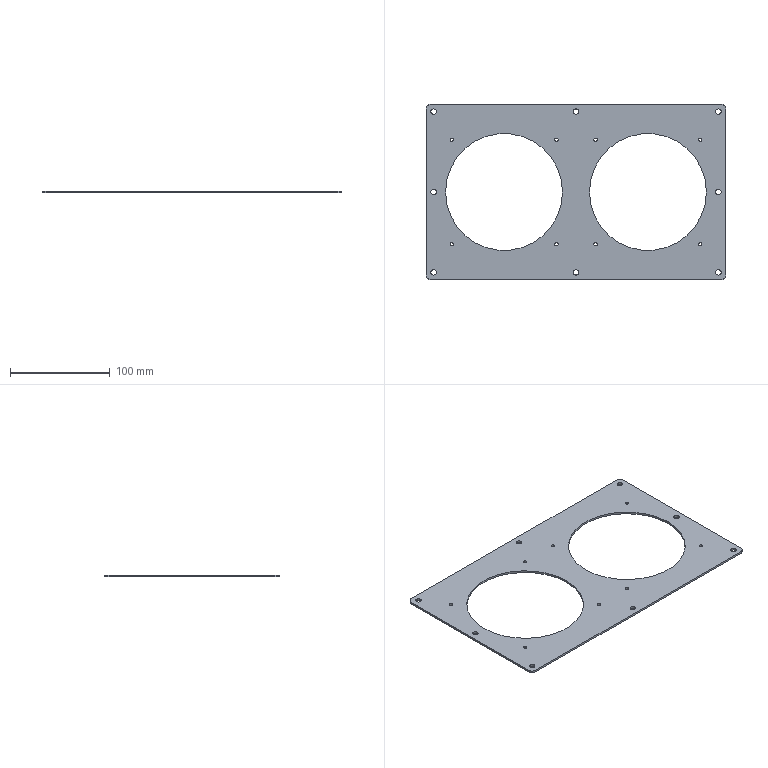Part | SolidWorks | features BaseBody 1 | 1 solid | 46 faces | box 300 x 176 x 2 mm | volume 62035 mm3 | cylinder 40 | plane 6 | commonest cylinder face diameters 3.3 x16 5.5 x16 10 x4 117 x4